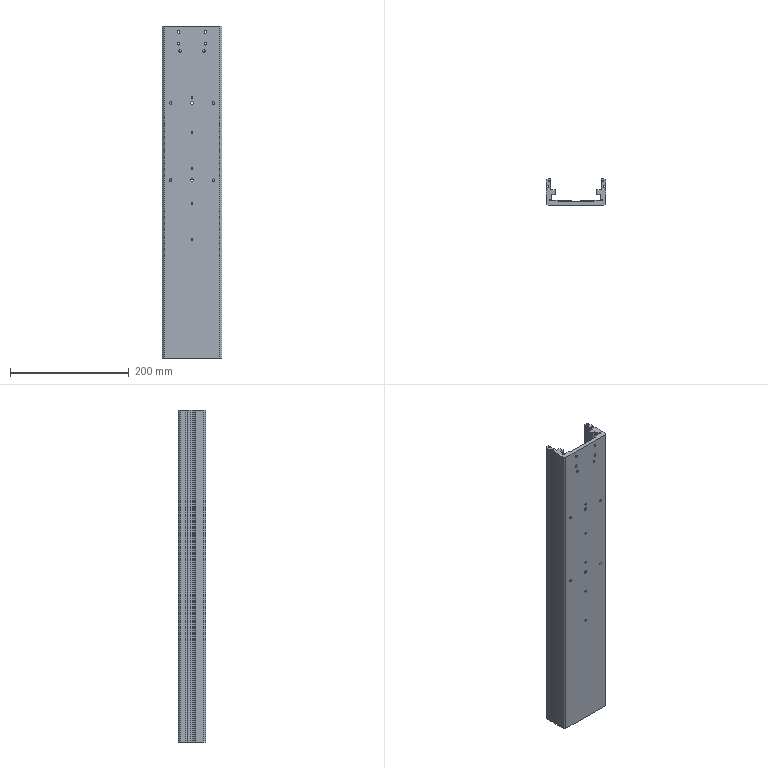Part | NX | 1 solid | 107 faces | box 100 x 46 x 560 mm | volume 769378 mm3 | plane 62 | cylinder 45 | commonest cylinder face diameters 0.6 x18 4.2 x10 3.3 x5 3.2 x4 0.4 x2 4 x2